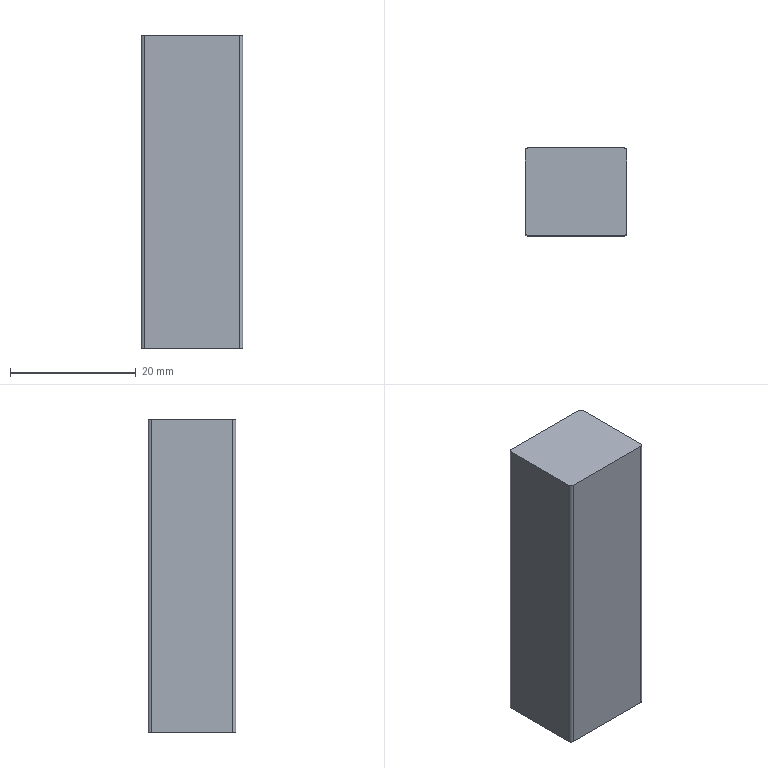Part | NX | features BREP 1 | 1 solid | 10 faces | box 16.163 x 13.999 x 50 mm | volume 11303 mm3 | plane 6 | cylinder 4 | commonest cylinder face diameters 1 x4
STEP:
#1=CARTESIAN_POINT('',(-7.581,7.,-40.6));
#2=VERTEX_POINT('',#1);
#3=CARTESIAN_POINT('',(-8.081,6.5,-40.6));
#4=VERTEX_POINT('',#3);
#5=CARTESIAN_POINT('',(-7.581,6.5,-40.6));
#6=DIRECTION('',(0.,0.,1.));
#7=DIRECTION('',(1.,0.,0.));
#8=AXIS2_PLACEMENT_3D('',#5,#6,#7);
#9=CIRCLE('',#8,0.5);
#10=EDGE_CURVE('',#2,#4,#9,.T.);
#11=ORIENTED_EDGE('',*,*,#10,.F.);
#12=CARTESIAN_POINT('',(-7.581,7.,-90.6));
#13=VERTEX_POINT('',#12);
#14=CARTESIAN_POINT('',(-7.581,7.,-90.6));
#15=DIRECTION('',(0.,0.,1.));
#16=VECTOR('',#15,1000.);
#17=LINE('',#14,#16);
#18=EDGE_CURVE('',#13,#2,#17,.T.);
#19=ORIENTED_EDGE('',*,*,#18,.F.);
#20=CARTESIAN_POINT('',(-8.081,6.5,-90.6));
#21=VERTEX_POINT('',#20);
#22=CARTESIAN_POINT('',(-7.581,6.5,-90.6));
#23=DIRECTION('',(0.,0.,1.));
#24=DIRECTION('',(1.,0.,0.));
#25=AXIS2_PLACEMENT_3D('',#22,#23,#24);
#26=CIRCLE('',#25,0.5);
#27=EDGE_CURVE('',#13,#21,#26,.T.);
#28=ORIENTED_EDGE('',*,*,#27,.T.);
#29=CARTESIAN_POINT('',(-8.081,6.5,-90.6));
#30=DIRECTION('',(0.,0.,1.));
#31=VECTOR('',#30,1000.);
#32=LINE('',#29,#31);
#33=EDGE_CURVE('',#21,#4,#32,.T.);
#34=ORIENTED_EDGE('',*,*,#33,.T.);
#35=EDGE_LOOP('',(#11,#19,#28,#34));
#36=FACE_BOUND('',#35,.T.);
#37=CARTESIAN_POINT('',(-7.581,6.5,-90.6));
#38=DIRECTION('',(0.,0.,1.));
#39=DIRECTION('',(-1.,0.,0.));
#40=AXIS2_PLACEMENT_3D('',#37,#38,#39);
#41=CYLINDRICAL_SURFACE('',#40,0.5);
#42=ADVANCED_FACE('',(#36),#41,.T.);
#43=CARTESIAN_POINT('',(-8.081,-6.5,-40.6));
#44=VERTEX_POINT('',#43);
#45=CARTESIAN_POINT('',(-8.081,-6.5,-40.6));
#46=DIRECTION('',(0.,1.,0.));
#47=VECTOR('',#46,1000.);
#48=LINE('',#45,#47);
#49=EDGE_CURVE('',#44,#4,#48,.T.);
#50=ORIENTED_EDGE('',*,*,#49,.T.);
#51=ORIENTED_EDGE('',*,*,#33,.F.);
#52=CARTESIAN_POINT('',(-8.081,-6.5,-90.6));
#53=VERTEX_POINT('',#52);
#54=CARTESIAN_POINT('',(-8.081,-6.5,-90.6));
#55=DIRECTION('',(0.,1.,0.));
#56=VECTOR('',#55,1000.);
#57=LINE('',#54,#56);
#58=EDGE_CURVE('',#53,#21,#57,.T.);
#59=ORIENTED_EDGE('',*,*,#58,.F.);
#60=CARTESIAN_POINT('',(-8.081,-6.5,-90.6));
#61=DIRECTION('',(0.,0.,1.));
#62=VECTOR('',#61,1000.);
#63=LINE('',#60,#62);
#64=EDGE_CURVE('',#53,#44,#63,.T.);
#65=ORIENTED_EDGE('',*,*,#64,.T.);
#66=EDGE_LOOP('',(#50,#51,#59,#65));
#67=FACE_BOUND('',#66,.T.);
#68=CARTESIAN_POINT('',(-8.081,-6.5,-90.6));
#69=DIRECTION('',(1.,0.,0.));
#70=DIRECTION('',(0.,0.,1.));
#71=AXIS2_PLACEMENT_3D('',#68,#69,#70);
#72=PLANE('',#71);
#73=ADVANCED_FACE('',(#67),#72,.F.);
#74=CARTESIAN_POINT('',(-7.581,-7.,-40.6));
#75=VERTEX_POINT('',#74);
#76=CARTESIAN_POINT('',(-7.581,-6.5,-40.6));
#77=DIRECTION('',(0.,0.,1.));
#78=DIRECTION('',(1.,0.,0.));
#79=AXIS2_PLACEMENT_3D('',#76,#77,#78);
#80=CIRCLE('',#79,0.5);
#81=EDGE_CURVE('',#44,#75,#80,.T.);
#82=ORIENTED_EDGE('',*,*,#81,.F.);
#83=ORIENTED_EDGE('',*,*,#64,.F.);
#84=CARTESIAN_POINT('',(-7.581,-7.,-90.6));
#85=VERTEX_POINT('',#84);
#86=CARTESIAN_POINT('',(-7.581,-6.5,-90.6));
#87=DIRECTION('',(0.,0.,1.));
#88=DIRECTION('',(1.,0.,0.));
#89=AXIS2_PLACEMENT_3D('',#86,#87,#88);
#90=CIRCLE('',#89,0.5);
#91=EDGE_CURVE('',#53,#85,#90,.T.);
#92=ORIENTED_EDGE('',*,*,#91,.T.);
#93=CARTESIAN_POINT('',(-7.581,-7.,-90.6));
#94=DIRECTION('',(0.,0.,1.));
#95=VECTOR('',#94,1000.);
#96=LINE('',#93,#95);
#97=EDGE_CURVE('',#85,#75,#96,.T.);
#98=ORIENTED_EDGE('',*,*,#97,.T.);
#99=EDGE_LOOP('',(#82,#83,#92,#98));
#100=FACE_BOUND('',#99,.T.);
#101=CARTESIAN_POINT('',(-7.581,-6.5,-90.6));
#102=DIRECTION('',(0.,0.,1.));
#103=DIRECTION('',(-1.,0.,0.));
#104=AXIS2_PLACEMENT_3D('',#101,#102,#103);
#105=CYLINDRICAL_SURFACE('',#104,0.5);
#106=ADVANCED_FACE('',(#100),#105,.T.);
#107=CARTESIAN_POINT('',(7.581,-7.,-40.6));
#108=VERTEX_POINT('',#107);
#109=CARTESIAN_POINT('',(7.581,-7.,-40.6));
#110=DIRECTION('',(-1.,0.,0.));
#111=VECTOR('',#110,1000.);
#112=LINE('',#109,#111);
#113=EDGE_CURVE('',#108,#75,#112,.T.);
#114=ORIENTED_EDGE('',*,*,#113,.T.);
#115=ORIENTED_EDGE('',*,*,#97,.F.);
#116=CARTESIAN_POINT('',(7.581,-7.,-90.6));
#117=VERTEX_POINT('',#116);
#118=CARTESIAN_POINT('',(7.581,-7.,-90.6));
#119=DIRECTION('',(-1.,0.,0.));
#120=VECTOR('',#119,1000.);
#121=LINE('',#118,#120);
#122=EDGE_CURVE('',#117,#85,#121,.T.);
#123=ORIENTED_EDGE('',*,*,#122,.F.);
#124=CARTESIAN_POINT('',(7.581,-7.,-90.6));
#125=DIRECTION('',(0.,0.,1.));
#126=VECTOR('',#125,1000.);
#127=LINE('',#124,#126);
#128=EDGE_CURVE('',#117,#108,#127,.T.);
#129=ORIENTED_EDGE('',*,*,#128,.T.);
#130=EDGE_LOOP('',(#114,#115,#123,#129));
#131=FACE_BOUND('',#130,.T.);
#132=CARTESIAN_POINT('',(7.581,-7.,-90.6));
#133=DIRECTION('',(0.,1.,0.));
#134=DIRECTION('',(0.,0.,-1.));
#135=AXIS2_PLACEMENT_3D('',#132,#133,#134);
#136=PLANE('',#135);
#137=ADVANCED_FACE('',(#131),#136,.F.);
#138=CARTESIAN_POINT('',(8.081,-6.5,-40.6));
#139=VERTEX_POINT('',#138);
#140=CARTESIAN_POINT('',(7.581,-6.5,-40.6));
#141=DIRECTION('',(0.,0.,1.));
#142=DIRECTION('',(1.,0.,0.));
#143=AXIS2_PLACEMENT_3D('',#140,#141,#142);
#144=CIRCLE('',#143,0.5);
#145=EDGE_CURVE('',#108,#139,#144,.T.);
#146=ORIENTED_EDGE('',*,*,#145,.F.);
#147=ORIENTED_EDGE('',*,*,#128,.F.);
#148=CARTESIAN_POINT('',(8.081,-6.5,-90.6));
#149=VERTEX_POINT('',#148);
#150=CARTESIAN_POINT('',(7.581,-6.5,-90.6));
#151=DIRECTION('',(0.,0.,1.));
#152=DIRECTION('',(1.,0.,0.));
#153=AXIS2_PLACEMENT_3D('',#150,#151,#152);
#154=CIRCLE('',#153,0.5);
#155=EDGE_CURVE('',#117,#149,#154,.T.);
#156=ORIENTED_EDGE('',*,*,#155,.T.);
#157=CARTESIAN_POINT('',(8.081,-6.5,-90.6));
#158=DIRECTION('',(0.,0.,1.));
#159=VECTOR('',#158,1000.);
#160=LINE('',#157,#159);
#161=EDGE_CURVE('',#149,#139,#160,.T.);
#162=ORIENTED_EDGE('',*,*,#161,.T.);
#163=EDGE_LOOP('',(#146,#147,#156,#162));
#164=FACE_BOUND('',#163,.T.);
#165=CARTESIAN_POINT('',(7.581,-6.5,-90.6));
#166=DIRECTION('',(0.,0.,1.));
#167=DIRECTION('',(-1.,0.,0.));
#168=AXIS2_PLACEMENT_3D('',#165,#166,#167);
#169=CYLINDRICAL_SURFACE('',#168,0.5);
#170=ADVANCED_FACE('',(#164),#169,.T.);
#171=CARTESIAN_POINT('',(8.081,6.5,-40.6));
#172=VERTEX_POINT('',#171);
#173=CARTESIAN_POINT('',(8.081,6.5,-40.6));
#174=DIRECTION('',(0.,-1.,0.));
#175=VECTOR('',#174,1000.);
#176=LINE('',#173,#175);
#177=EDGE_CURVE('',#172,#139,#176,.T.);
#178=ORIENTED_EDGE('',*,*,#177,.T.);
#179=ORIENTED_EDGE('',*,*,#161,.F.);
#180=CARTESIAN_POINT('',(8.081,6.5,-90.6));
#181=VERTEX_POINT('',#180);
#182=CARTESIAN_POINT('',(8.081,6.5,-90.6));
#183=DIRECTION('',(0.,-1.,0.));
#184=VECTOR('',#183,1000.);
#185=LINE('',#182,#184);
#186=EDGE_CURVE('',#181,#149,#185,.T.);
#187=ORIENTED_EDGE('',*,*,#186,.F.);
#188=CARTESIAN_POINT('',(8.081,6.5,-90.6));
#189=DIRECTION('',(0.,0.,1.));
#190=VECTOR('',#189,1000.);
#191=LINE('',#188,#190);
#192=EDGE_CURVE('',#181,#172,#191,.T.);
#193=ORIENTED_EDGE('',*,*,#192,.T.);
#194=EDGE_LOOP('',(#178,#179,#187,#193));
#195=FACE_BOUND('',#194,.T.);
#196=CARTESIAN_POINT('',(8.081,6.5,-90.6));
#197=DIRECTION('',(-1.,0.,0.));
#198=DIRECTION('',(0.,1.,0.));
#199=AXIS2_PLACEMENT_3D('',#196,#197,#198);
#200=PLANE('',#199);
#201=ADVANCED_FACE('',(#195),#200,.F.);
#202=CARTESIAN_POINT('',(7.581,7.,-40.6));
#203=VERTEX_POINT('',#202);
#204=CARTESIAN_POINT('',(7.581,6.5,-40.6));
#205=DIRECTION('',(0.,0.,1.));
#206=DIRECTION('',(1.,0.,0.));
#207=AXIS2_PLACEMENT_3D('',#204,#205,#206);
#208=CIRCLE('',#207,0.5);
#209=EDGE_CURVE('',#172,#203,#208,.T.);
#210=ORIENTED_EDGE('',*,*,#209,.F.);
#211=ORIENTED_EDGE('',*,*,#192,.F.);
#212=CARTESIAN_POINT('',(7.581,7.,-90.6));
#213=VERTEX_POINT('',#212);
#214=CARTESIAN_POINT('',(7.581,6.5,-90.6));
#215=DIRECTION('',(0.,0.,1.));
#216=DIRECTION('',(1.,0.,0.));
#217=AXIS2_PLACEMENT_3D('',#214,#215,#216);
#218=CIRCLE('',#217,0.5);
#219=EDGE_CURVE('',#181,#213,#218,.T.);
#220=ORIENTED_EDGE('',*,*,#219,.T.);
#221=CARTESIAN_POINT('',(7.581,7.,-90.6));
#222=DIRECTION('',(0.,0.,1.));
#223=VECTOR('',#222,1000.);
#224=LINE('',#221,#223);
#225=EDGE_CURVE('',#213,#203,#224,.T.);
#226=ORIENTED_EDGE('',*,*,#225,.T.);
#227=EDGE_LOOP('',(#210,#211,#220,#226));
#228=FACE_BOUND('',#227,.T.);
#229=CARTESIAN_POINT('',(7.581,6.5,-90.6));
#230=DIRECTION('',(0.,0.,1.));
#231=DIRECTION('',(-1.,0.,0.));
#232=AXIS2_PLACEMENT_3D('',#229,#230,#231);
#233=CYLINDRICAL_SURFACE('',#232,0.5);
#234=ADVANCED_FACE('',(#228),#233,.T.);
#235=CARTESIAN_POINT('',(-7.581,7.,-40.6));
#236=DIRECTION('',(1.,0.,0.));
#237=VECTOR('',#236,1000.);
#238=LINE('',#235,#237);
#239=EDGE_CURVE('',#2,#203,#238,.T.);
#240=ORIENTED_EDGE('',*,*,#239,.T.);
#241=ORIENTED_EDGE('',*,*,#225,.F.);
#242=CARTESIAN_POINT('',(-7.581,7.,-90.6));
#243=DIRECTION('',(1.,0.,0.));
#244=VECTOR('',#243,1000.);
#245=LINE('',#242,#244);
#246=EDGE_CURVE('',#13,#213,#245,.T.);
#247=ORIENTED_EDGE('',*,*,#246,.F.);
#248=ORIENTED_EDGE('',*,*,#18,.T.);
#249=EDGE_LOOP('',(#240,#241,#247,#248));
#250=FACE_BOUND('',#249,.T.);
#251=CARTESIAN_POINT('',(-7.581,7.,-90.6));
#252=DIRECTION('',(0.,-1.,0.));
#253=DIRECTION('',(0.,0.,1.));
#254=AXIS2_PLACEMENT_3D('',#251,#252,#253);
#255=PLANE('',#254);
#256=ADVANCED_FACE('',(#250),#255,.F.);
#257=ORIENTED_EDGE('',*,*,#27,.F.);
#258=ORIENTED_EDGE('',*,*,#246,.T.);
#259=ORIENTED_EDGE('',*,*,#219,.F.);
#260=ORIENTED_EDGE('',*,*,#186,.T.);
#261=ORIENTED_EDGE('',*,*,#155,.F.);
#262=ORIENTED_EDGE('',*,*,#122,.T.);
#263=ORIENTED_EDGE('',*,*,#91,.F.);
#264=ORIENTED_EDGE('',*,*,#58,.T.);
#265=EDGE_LOOP('',(#257,#258,#259,#260,#261,#262,#263,#264));
#266=FACE_BOUND('',#265,.T.);
#267=CARTESIAN_POINT('',(-7.581,6.5,-90.6));
#268=DIRECTION('',(0.,0.,1.));
#269=DIRECTION('',(-1.,0.,0.));
#270=AXIS2_PLACEMENT_3D('',#267,#268,#269);
#271=PLANE('',#270);
#272=ADVANCED_FACE('',(#266),#271,.F.);
#273=ORIENTED_EDGE('',*,*,#10,.T.);
#274=ORIENTED_EDGE('',*,*,#49,.F.);
#275=ORIENTED_EDGE('',*,*,#81,.T.);
#276=ORIENTED_EDGE('',*,*,#113,.F.);
#277=ORIENTED_EDGE('',*,*,#145,.T.);
#278=ORIENTED_EDGE('',*,*,#177,.F.);
#279=ORIENTED_EDGE('',*,*,#209,.T.);
#280=ORIENTED_EDGE('',*,*,#239,.F.);
#281=EDGE_LOOP('',(#273,#274,#275,#276,#277,#278,#279,#280));
#282=FACE_BOUND('',#281,.T.);
#283=CARTESIAN_POINT('',(-7.581,6.5,-40.6));
#284=DIRECTION('',(0.,0.,1.));
#285=DIRECTION('',(-1.,0.,0.));
#286=AXIS2_PLACEMENT_3D('',#283,#284,#285);
#287=PLANE('',#286);
#288=ADVANCED_FACE('',(#282),#287,.T.);
#289=CLOSED_SHELL('',(#42,#73,#106,#137,#170,#201,#234,#256,#272,#288));
#290=MANIFOLD_SOLID_BREP('',#289);
#291=(LENGTH_UNIT()NAMED_UNIT(*)SI_UNIT(.MILLI.,.METRE.));
#292=UNCERTAINTY_MEASURE_WITH_UNIT(LENGTH_MEASURE(0.00001),#291,'','');
#293=(NAMED_UNIT(*)PLANE_ANGLE_UNIT()SI_UNIT($,.RADIAN.));
#294=(NAMED_UNIT(*)SI_UNIT($,.STERADIAN.)SOLID_ANGLE_UNIT());
#295=(GEOMETRIC_REPRESENTATION_CONTEXT(3)GLOBAL_UNCERTAINTY_ASSIGNED_CONTEXT((#292))GLOBAL_UNIT_ASSIGNED_CONTEXT((#291,#293,#294))REPRESENTATION_CONTEXT('',''));
#296=ADVANCED_BREP_SHAPE_REPRESENTATION('',(#290),#295);